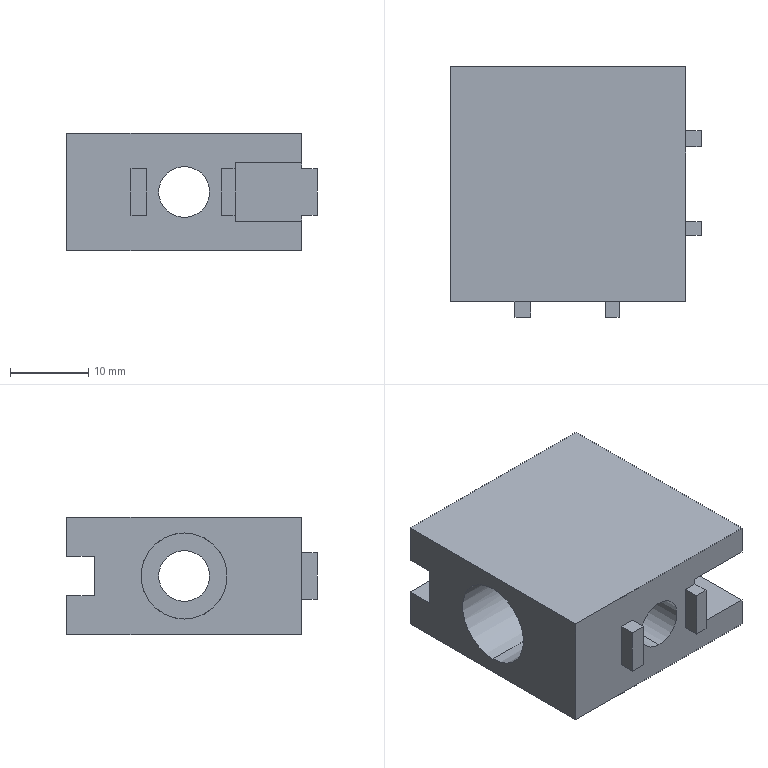Part | NX | features BREP 1 | 1 solid | 49 faces | box 32 x 32 x 15 mm | volume 8511 mm3 | plane 37 | cylinder 12 | commonest cylinder face diameters 11 x8 6.5 x4
STEP:
#1=CARTESIAN_POINT('',(0.,0.,5.5));
#2=VERTEX_POINT('',#1);
#3=CARTESIAN_POINT('',(0.,0.,-5.5));
#4=VERTEX_POINT('',#3);
#5=CARTESIAN_POINT('',(0.,0.,5.5));
#6=CARTESIAN_POINT('',(-11.,-11.,5.5));
#7=CARTESIAN_POINT('',(-11.,-11.,-5.5));
#8=CARTESIAN_POINT('',(0.,0.,-5.5));
#9=(BOUNDED_CURVE()B_SPLINE_CURVE(3,(#5,#6,#7,#8),.UNSPECIFIED.,.F.,.F.)B_SPLINE_CURVE_WITH_KNOTS((4,4),(4.712,7.854),.UNSPECIFIED.)CURVE()GEOMETRIC_REPRESENTATION_ITEM()RATIONAL_B_SPLINE_CURVE((1.,0.3333,0.3333,1.))REPRESENTATION_ITEM(''));
#10=EDGE_CURVE('',#2,#4,#9,.T.);
#11=ORIENTED_EDGE('',*,*,#10,.T.);
#12=CARTESIAN_POINT('',(-15.,0.,-5.5));
#13=VERTEX_POINT('',#12);
#14=CARTESIAN_POINT('',(0.,0.,-5.5));
#15=DIRECTION('',(-1.,0.,0.));
#16=VECTOR('',#15,1000.);
#17=LINE('',#14,#16);
#18=EDGE_CURVE('',#13,#4,#17,.F.);
#19=ORIENTED_EDGE('',*,*,#18,.F.);
#20=CARTESIAN_POINT('',(-15.,0.,5.5));
#21=VERTEX_POINT('',#20);
#22=CARTESIAN_POINT('',(-15.,0.,0.));
#23=DIRECTION('',(-1.,0.,0.));
#24=DIRECTION('',(0.,0.,1.));
#25=AXIS2_PLACEMENT_3D('',#22,#23,#24);
#26=CIRCLE('',#25,5.5);
#27=EDGE_CURVE('',#13,#21,#26,.T.);
#28=ORIENTED_EDGE('',*,*,#27,.T.);
#29=CARTESIAN_POINT('',(0.,0.,5.5));
#30=DIRECTION('',(-1.,0.,0.));
#31=VECTOR('',#30,1000.);
#32=LINE('',#29,#31);
#33=EDGE_CURVE('',#21,#2,#32,.F.);
#34=ORIENTED_EDGE('',*,*,#33,.T.);
#35=EDGE_LOOP('',(#11,#19,#28,#34));
#36=FACE_BOUND('',#35,.T.);
#37=CARTESIAN_POINT('',(0.,0.,0.));
#38=DIRECTION('',(-1.,0.,0.));
#39=DIRECTION('',(0.,0.,1.));
#40=AXIS2_PLACEMENT_3D('',#37,#38,#39);
#41=CYLINDRICAL_SURFACE('',#40,5.5);
#42=ADVANCED_FACE('',(#36),#41,.F.);
#43=CARTESIAN_POINT('',(10.,0.,-5.5));
#44=VERTEX_POINT('',#43);
#45=CARTESIAN_POINT('',(10.,0.,5.5));
#46=VERTEX_POINT('',#45);
#47=CARTESIAN_POINT('',(10.,0.,0.));
#48=DIRECTION('',(-1.,0.,0.));
#49=DIRECTION('',(0.,0.,1.));
#50=AXIS2_PLACEMENT_3D('',#47,#48,#49);
#51=CIRCLE('',#50,5.5);
#52=EDGE_CURVE('',#44,#46,#51,.T.);
#53=ORIENTED_EDGE('',*,*,#52,.F.);
#54=CARTESIAN_POINT('',(0.,0.,-5.5));
#55=DIRECTION('',(-1.,0.,0.));
#56=VECTOR('',#55,1000.);
#57=LINE('',#54,#56);
#58=EDGE_CURVE('',#4,#44,#57,.F.);
#59=ORIENTED_EDGE('',*,*,#58,.F.);
#60=CARTESIAN_POINT('',(0.,0.,-5.5));
#61=CARTESIAN_POINT('',(11.,-11.,-5.5));
#62=CARTESIAN_POINT('',(11.,-11.,5.5));
#63=CARTESIAN_POINT('',(0.,0.,5.5));
#64=(BOUNDED_CURVE()B_SPLINE_CURVE(3,(#60,#61,#62,#63),.UNSPECIFIED.,.F.,.F.)B_SPLINE_CURVE_WITH_KNOTS((4,4),(4.712,7.854),.UNSPECIFIED.)CURVE()GEOMETRIC_REPRESENTATION_ITEM()RATIONAL_B_SPLINE_CURVE((1.,0.3333,0.3333,1.))REPRESENTATION_ITEM(''));
#65=EDGE_CURVE('',#4,#2,#64,.T.);
#66=ORIENTED_EDGE('',*,*,#65,.T.);
#67=CARTESIAN_POINT('',(0.,0.,5.5));
#68=DIRECTION('',(-1.,0.,0.));
#69=VECTOR('',#68,1000.);
#70=LINE('',#67,#69);
#71=EDGE_CURVE('',#2,#46,#70,.F.);
#72=ORIENTED_EDGE('',*,*,#71,.T.);
#73=EDGE_LOOP('',(#53,#59,#66,#72));
#74=FACE_BOUND('',#73,.T.);
#75=CARTESIAN_POINT('',(0.,0.,0.));
#76=DIRECTION('',(-1.,0.,0.));
#77=DIRECTION('',(0.,0.,1.));
#78=AXIS2_PLACEMENT_3D('',#75,#76,#77);
#79=CYLINDRICAL_SURFACE('',#78,5.5);
#80=ADVANCED_FACE('',(#74),#79,.F.);
#81=CARTESIAN_POINT('',(15.,0.,-3.25));
#82=VERTEX_POINT('',#81);
#83=CARTESIAN_POINT('',(15.,0.,3.25));
#84=VERTEX_POINT('',#83);
#85=CARTESIAN_POINT('',(15.,0.,0.));
#86=DIRECTION('',(-1.,0.,0.));
#87=DIRECTION('',(0.,0.,1.));
#88=AXIS2_PLACEMENT_3D('',#85,#86,#87);
#89=CIRCLE('',#88,3.25);
#90=EDGE_CURVE('',#82,#84,#89,.T.);
#91=ORIENTED_EDGE('',*,*,#90,.F.);
#92=CARTESIAN_POINT('',(10.,0.,-3.25));
#93=VERTEX_POINT('',#92);
#94=CARTESIAN_POINT('',(0.,0.,-3.25));
#95=DIRECTION('',(-1.,0.,0.));
#96=VECTOR('',#95,1000.);
#97=LINE('',#94,#96);
#98=EDGE_CURVE('',#93,#82,#97,.F.);
#99=ORIENTED_EDGE('',*,*,#98,.F.);
#100=CARTESIAN_POINT('',(10.,0.,3.25));
#101=VERTEX_POINT('',#100);
#102=CARTESIAN_POINT('',(10.,0.,0.));
#103=DIRECTION('',(-1.,0.,0.));
#104=DIRECTION('',(0.,0.,1.));
#105=AXIS2_PLACEMENT_3D('',#102,#103,#104);
#106=CIRCLE('',#105,3.25);
#107=EDGE_CURVE('',#93,#101,#106,.T.);
#108=ORIENTED_EDGE('',*,*,#107,.T.);
#109=CARTESIAN_POINT('',(0.,0.,3.25));
#110=DIRECTION('',(-1.,0.,0.));
#111=VECTOR('',#110,1000.);
#112=LINE('',#109,#111);
#113=EDGE_CURVE('',#101,#84,#112,.F.);
#114=ORIENTED_EDGE('',*,*,#113,.T.);
#115=EDGE_LOOP('',(#91,#99,#108,#114));
#116=FACE_BOUND('',#115,.T.);
#117=CARTESIAN_POINT('',(0.,0.,0.));
#118=DIRECTION('',(-1.,0.,0.));
#119=DIRECTION('',(0.,0.,1.));
#120=AXIS2_PLACEMENT_3D('',#117,#118,#119);
#121=CYLINDRICAL_SURFACE('',#120,3.25);
#122=ADVANCED_FACE('',(#116),#121,.F.);
#123=CARTESIAN_POINT('',(0.,-10.,3.25));
#124=VERTEX_POINT('',#123);
#125=CARTESIAN_POINT('',(0.,-10.,-3.25));
#126=VERTEX_POINT('',#125);
#127=CARTESIAN_POINT('',(0.,-10.,0.));
#128=DIRECTION('',(0.,-1.,0.));
#129=DIRECTION('',(0.,0.,-1.));
#130=AXIS2_PLACEMENT_3D('',#127,#128,#129);
#131=CIRCLE('',#130,3.25);
#132=EDGE_CURVE('',#124,#126,#131,.T.);
#133=ORIENTED_EDGE('',*,*,#132,.F.);
#134=CARTESIAN_POINT('',(0.,-15.,3.25));
#135=VERTEX_POINT('',#134);
#136=CARTESIAN_POINT('',(0.,0.,3.25));
#137=DIRECTION('',(0.,-1.,0.));
#138=VECTOR('',#137,1000.);
#139=LINE('',#136,#138);
#140=EDGE_CURVE('',#124,#135,#139,.T.);
#141=ORIENTED_EDGE('',*,*,#140,.T.);
#142=CARTESIAN_POINT('',(0.,-15.,-3.25));
#143=VERTEX_POINT('',#142);
#144=CARTESIAN_POINT('',(0.,-15.,0.));
#145=DIRECTION('',(0.,-1.,0.));
#146=DIRECTION('',(0.,0.,-1.));
#147=AXIS2_PLACEMENT_3D('',#144,#145,#146);
#148=CIRCLE('',#147,3.25);
#149=EDGE_CURVE('',#135,#143,#148,.T.);
#150=ORIENTED_EDGE('',*,*,#149,.T.);
#151=CARTESIAN_POINT('',(0.,0.,-3.25));
#152=DIRECTION('',(0.,-1.,0.));
#153=VECTOR('',#152,1000.);
#154=LINE('',#151,#153);
#155=EDGE_CURVE('',#126,#143,#154,.T.);
#156=ORIENTED_EDGE('',*,*,#155,.F.);
#157=EDGE_LOOP('',(#133,#141,#150,#156));
#158=FACE_BOUND('',#157,.T.);
#159=CARTESIAN_POINT('',(0.,0.,0.));
#160=DIRECTION('',(0.,-1.,0.));
#161=DIRECTION('',(0.,0.,-1.));
#162=AXIS2_PLACEMENT_3D('',#159,#160,#161);
#163=CYLINDRICAL_SURFACE('',#162,3.25);
#164=ADVANCED_FACE('',(#158),#163,.F.);
#165=ORIENTED_EDGE('',*,*,#10,.F.);
#166=CARTESIAN_POINT('',(0.,-10.,5.5));
#167=VERTEX_POINT('',#166);
#168=CARTESIAN_POINT('',(0.,0.,5.5));
#169=DIRECTION('',(0.,-1.,0.));
#170=VECTOR('',#169,1000.);
#171=LINE('',#168,#170);
#172=EDGE_CURVE('',#2,#167,#171,.T.);
#173=ORIENTED_EDGE('',*,*,#172,.T.);
#174=CARTESIAN_POINT('',(0.,-10.,-5.5));
#175=VERTEX_POINT('',#174);
#176=CARTESIAN_POINT('',(0.,-10.,0.));
#177=DIRECTION('',(0.,-1.,0.));
#178=DIRECTION('',(0.,0.,-1.));
#179=AXIS2_PLACEMENT_3D('',#176,#177,#178);
#180=CIRCLE('',#179,5.5);
#181=EDGE_CURVE('',#167,#175,#180,.T.);
#182=ORIENTED_EDGE('',*,*,#181,.T.);
#183=CARTESIAN_POINT('',(0.,0.,-5.5));
#184=DIRECTION('',(0.,-1.,0.));
#185=VECTOR('',#184,1000.);
#186=LINE('',#183,#185);
#187=EDGE_CURVE('',#4,#175,#186,.T.);
#188=ORIENTED_EDGE('',*,*,#187,.F.);
#189=EDGE_LOOP('',(#165,#173,#182,#188));
#190=FACE_BOUND('',#189,.T.);
#191=CARTESIAN_POINT('',(0.,0.,0.));
#192=DIRECTION('',(0.,-1.,0.));
#193=DIRECTION('',(0.,0.,-1.));
#194=AXIS2_PLACEMENT_3D('',#191,#192,#193);
#195=CYLINDRICAL_SURFACE('',#194,5.5);
#196=ADVANCED_FACE('',(#190),#195,.F.);
#197=CARTESIAN_POINT('',(0.,15.,5.5));
#198=VERTEX_POINT('',#197);
#199=CARTESIAN_POINT('',(-4.899,15.,2.5));
#200=VERTEX_POINT('',#199);
#201=CARTESIAN_POINT('',(0.,15.,0.));
#202=DIRECTION('',(0.,-1.,0.));
#203=DIRECTION('',(0.,0.,-1.));
#204=AXIS2_PLACEMENT_3D('',#201,#202,#203);
#205=CIRCLE('',#204,5.5);
#206=EDGE_CURVE('',#198,#200,#205,.T.);
#207=ORIENTED_EDGE('',*,*,#206,.F.);
#208=CARTESIAN_POINT('',(0.,0.,5.5));
#209=DIRECTION('',(0.,-1.,0.));
#210=VECTOR('',#209,1000.);
#211=LINE('',#208,#210);
#212=EDGE_CURVE('',#198,#2,#211,.T.);
#213=ORIENTED_EDGE('',*,*,#212,.T.);
#214=CARTESIAN_POINT('',(0.,0.,-5.5));
#215=CARTESIAN_POINT('',(-11.,11.,-5.5));
#216=CARTESIAN_POINT('',(-11.,11.,5.5));
#217=CARTESIAN_POINT('',(0.,0.,5.5));
#218=(BOUNDED_CURVE()B_SPLINE_CURVE(3,(#214,#215,#216,#217),.UNSPECIFIED.,.F.,.F.)B_SPLINE_CURVE_WITH_KNOTS((4,4),(1.571,4.712),.UNSPECIFIED.)CURVE()GEOMETRIC_REPRESENTATION_ITEM()RATIONAL_B_SPLINE_CURVE((1.,0.3333,0.3333,1.))REPRESENTATION_ITEM(''));
#219=EDGE_CURVE('',#4,#2,#218,.T.);
#220=ORIENTED_EDGE('',*,*,#219,.F.);
#221=CARTESIAN_POINT('',(0.,15.,-5.5));
#222=VERTEX_POINT('',#221);
#223=CARTESIAN_POINT('',(0.,0.,-5.5));
#224=DIRECTION('',(0.,-1.,0.));
#225=VECTOR('',#224,1000.);
#226=LINE('',#223,#225);
#227=EDGE_CURVE('',#222,#4,#226,.T.);
#228=ORIENTED_EDGE('',*,*,#227,.F.);
#229=CARTESIAN_POINT('',(-4.899,15.,-2.5));
#230=VERTEX_POINT('',#229);
#231=CARTESIAN_POINT('',(0.,15.,0.));
#232=DIRECTION('',(0.,-1.,0.));
#233=DIRECTION('',(0.,0.,-1.));
#234=AXIS2_PLACEMENT_3D('',#231,#232,#233);
#235=CIRCLE('',#234,5.5);
#236=EDGE_CURVE('',#230,#222,#235,.T.);
#237=ORIENTED_EDGE('',*,*,#236,.F.);
#238=CARTESIAN_POINT('',(-4.899,11.5,-2.5));
#239=VERTEX_POINT('',#238);
#240=CARTESIAN_POINT('',(-4.899,0.,-2.5));
#241=DIRECTION('',(0.,-1.,0.));
#242=VECTOR('',#241,1000.);
#243=LINE('',#240,#242);
#244=EDGE_CURVE('',#230,#239,#243,.T.);
#245=ORIENTED_EDGE('',*,*,#244,.T.);
#246=CARTESIAN_POINT('',(-4.899,11.5,2.5));
#247=VERTEX_POINT('',#246);
#248=CARTESIAN_POINT('',(0.,11.5,0.));
#249=DIRECTION('',(0.,1.,0.));
#250=DIRECTION('',(0.,0.,-1.));
#251=AXIS2_PLACEMENT_3D('',#248,#249,#250);
#252=CIRCLE('',#251,5.5);
#253=EDGE_CURVE('',#239,#247,#252,.T.);
#254=ORIENTED_EDGE('',*,*,#253,.T.);
#255=CARTESIAN_POINT('',(-4.899,0.,2.5));
#256=DIRECTION('',(0.,1.,0.));
#257=VECTOR('',#256,1000.);
#258=LINE('',#255,#257);
#259=EDGE_CURVE('',#247,#200,#258,.T.);
#260=ORIENTED_EDGE('',*,*,#259,.T.);
#261=EDGE_LOOP('',(#207,#213,#220,#228,#237,#245,#254,#260));
#262=FACE_BOUND('',#261,.T.);
#263=CARTESIAN_POINT('',(0.,0.,0.));
#264=DIRECTION('',(0.,-1.,0.));
#265=DIRECTION('',(0.,0.,-1.));
#266=AXIS2_PLACEMENT_3D('',#263,#264,#265);
#267=CYLINDRICAL_SURFACE('',#266,5.5);
#268=ADVANCED_FACE('',(#262),#267,.F.);
#269=CARTESIAN_POINT('',(-15.,15.,2.5));
#270=VERTEX_POINT('',#269);
#271=CARTESIAN_POINT('',(-15.,15.,2.5));
#272=DIRECTION('',(1.,0.,0.));
#273=VECTOR('',#272,1000.);
#274=LINE('',#271,#273);
#275=EDGE_CURVE('',#270,#200,#274,.T.);
#276=ORIENTED_EDGE('',*,*,#275,.F.);
#277=CARTESIAN_POINT('',(-15.,15.,7.5));
#278=VERTEX_POINT('',#277);
#279=CARTESIAN_POINT('',(-15.,15.,-7.5));
#280=DIRECTION('',(0.,0.,1.));
#281=VECTOR('',#280,1000.);
#282=LINE('',#279,#281);
#283=EDGE_CURVE('',#270,#278,#282,.T.);
#284=ORIENTED_EDGE('',*,*,#283,.T.);
#285=CARTESIAN_POINT('',(15.,15.,7.5));
#286=VERTEX_POINT('',#285);
#287=CARTESIAN_POINT('',(-15.,15.,7.5));
#288=DIRECTION('',(-1.,0.,0.));
#289=VECTOR('',#288,1000.);
#290=LINE('',#287,#289);
#291=EDGE_CURVE('',#286,#278,#290,.T.);
#292=ORIENTED_EDGE('',*,*,#291,.F.);
#293=CARTESIAN_POINT('',(15.,15.,2.5));
#294=VERTEX_POINT('',#293);
#295=CARTESIAN_POINT('',(15.,15.,-7.5));
#296=DIRECTION('',(0.,0.,1.));
#297=VECTOR('',#296,1000.);
#298=LINE('',#295,#297);
#299=EDGE_CURVE('',#294,#286,#298,.T.);
#300=ORIENTED_EDGE('',*,*,#299,.F.);
#301=CARTESIAN_POINT('',(4.899,15.,2.5));
#302=VERTEX_POINT('',#301);
#303=CARTESIAN_POINT('',(-15.,15.,2.5));
#304=DIRECTION('',(1.,0.,0.));
#305=VECTOR('',#304,1000.);
#306=LINE('',#303,#305);
#307=EDGE_CURVE('',#302,#294,#306,.T.);
#308=ORIENTED_EDGE('',*,*,#307,.F.);
#309=CARTESIAN_POINT('',(0.,15.,0.));
#310=DIRECTION('',(0.,-1.,0.));
#311=DIRECTION('',(0.,0.,-1.));
#312=AXIS2_PLACEMENT_3D('',#309,#310,#311);
#313=CIRCLE('',#312,5.5);
#314=EDGE_CURVE('',#302,#198,#313,.T.);
#315=ORIENTED_EDGE('',*,*,#314,.T.);
#316=ORIENTED_EDGE('',*,*,#206,.T.);
#317=EDGE_LOOP('',(#276,#284,#292,#300,#308,#315,#316));
#318=FACE_BOUND('',#317,.T.);
#319=CARTESIAN_POINT('',(-15.,15.,-7.5));
#320=DIRECTION('',(0.,1.,0.));
#321=DIRECTION('',(1.,0.,0.));
#322=AXIS2_PLACEMENT_3D('',#319,#320,#321);
#323=PLANE('',#322);
#324=ADVANCED_FACE('',(#318),#323,.T.);
#325=CARTESIAN_POINT('',(15.,-6.5,-3.75));
#326=VERTEX_POINT('',#325);
#327=CARTESIAN_POINT('',(15.,-6.5,-3.));
#328=VERTEX_POINT('',#327);
#329=CARTESIAN_POINT('',(15.,-6.5,-3.75));
#330=DIRECTION('',(0.,0.,1.));
#331=VECTOR('',#330,1000.);
#332=LINE('',#329,#331);
#333=EDGE_CURVE('',#326,#328,#332,.T.);
#334=ORIENTED_EDGE('',*,*,#333,.F.);
#335=CARTESIAN_POINT('',(15.,-15.,-3.75));
#336=VERTEX_POINT('',#335);
#337=CARTESIAN_POINT('',(15.,-6.5,-3.75));
#338=DIRECTION('',(0.,1.,0.));
#339=VECTOR('',#338,1000.);
#340=LINE('',#337,#339);
#341=EDGE_CURVE('',#336,#326,#340,.T.);
#342=ORIENTED_EDGE('',*,*,#341,.F.);
#343=CARTESIAN_POINT('',(15.,-15.,-7.5));
#344=VERTEX_POINT('',#343);
#345=CARTESIAN_POINT('',(15.,-15.,-7.5));
#346=DIRECTION('',(0.,0.,1.));
#347=VECTOR('',#346,1000.);
#348=LINE('',#345,#347);
#349=EDGE_CURVE('',#344,#336,#348,.T.);
#350=ORIENTED_EDGE('',*,*,#349,.F.);
#351=CARTESIAN_POINT('',(15.,15.,-7.5));
#352=VERTEX_POINT('',#351);
#353=CARTESIAN_POINT('',(15.,-15.,-7.5));
#354=DIRECTION('',(0.,1.,0.));
#355=VECTOR('',#354,1000.);
#356=LINE('',#353,#355);
#357=EDGE_CURVE('',#344,#352,#356,.T.);
#358=ORIENTED_EDGE('',*,*,#357,.T.);
#359=CARTESIAN_POINT('',(15.,15.,-2.5));
#360=VERTEX_POINT('',#359);
#361=CARTESIAN_POINT('',(15.,15.,-7.5));
#362=DIRECTION('',(0.,0.,1.));
#363=VECTOR('',#362,1000.);
#364=LINE('',#361,#363);
#365=EDGE_CURVE('',#352,#360,#364,.T.);
#366=ORIENTED_EDGE('',*,*,#365,.T.);
#367=CARTESIAN_POINT('',(15.,11.5,-2.5));
#368=VERTEX_POINT('',#367);
#369=CARTESIAN_POINT('',(15.,-15.,-2.5));
#370=DIRECTION('',(0.,1.,0.));
#371=VECTOR('',#370,1000.);
#372=LINE('',#369,#371);
#373=EDGE_CURVE('',#368,#360,#372,.T.);
#374=ORIENTED_EDGE('',*,*,#373,.F.);
#375=CARTESIAN_POINT('',(15.,11.5,2.5));
#376=VERTEX_POINT('',#375);
#377=CARTESIAN_POINT('',(15.,11.5,-7.5));
#378=DIRECTION('',(0.,0.,-1.));
#379=VECTOR('',#378,1000.);
#380=LINE('',#377,#379);
#381=EDGE_CURVE('',#376,#368,#380,.T.);
#382=ORIENTED_EDGE('',*,*,#381,.F.);
#383=CARTESIAN_POINT('',(15.,-15.,2.5));
#384=DIRECTION('',(0.,-1.,0.));
#385=VECTOR('',#384,1000.);
#386=LINE('',#383,#385);
#387=EDGE_CURVE('',#294,#376,#386,.T.);
#388=ORIENTED_EDGE('',*,*,#387,.F.);
#389=ORIENTED_EDGE('',*,*,#299,.T.);
#390=CARTESIAN_POINT('',(15.,-15.,7.5));
#391=VERTEX_POINT('',#390);
#392=CARTESIAN_POINT('',(15.,-15.,7.5));
#393=DIRECTION('',(0.,1.,0.));
#394=VECTOR('',#393,1000.);
#395=LINE('',#392,#394);
#396=EDGE_CURVE('',#391,#286,#395,.T.);
#397=ORIENTED_EDGE('',*,*,#396,.F.);
#398=CARTESIAN_POINT('',(15.,-15.,3.75));
#399=VERTEX_POINT('',#398);
#400=CARTESIAN_POINT('',(15.,-15.,-7.5));
#401=DIRECTION('',(0.,0.,1.));
#402=VECTOR('',#401,1000.);
#403=LINE('',#400,#402);
#404=EDGE_CURVE('',#399,#391,#403,.T.);
#405=ORIENTED_EDGE('',*,*,#404,.F.);
#406=CARTESIAN_POINT('',(15.,-6.5,3.75));
#407=VERTEX_POINT('',#406);
#408=CARTESIAN_POINT('',(15.,-6.5,3.75));
#409=DIRECTION('',(0.,1.,0.));
#410=VECTOR('',#409,1000.);
#411=LINE('',#408,#410);
#412=EDGE_CURVE('',#399,#407,#411,.T.);
#413=ORIENTED_EDGE('',*,*,#412,.T.);
#414=CARTESIAN_POINT('',(15.,-6.5,3.));
#415=VERTEX_POINT('',#414);
#416=CARTESIAN_POINT('',(15.,-6.5,-3.75));
#417=DIRECTION('',(0.,0.,1.));
#418=VECTOR('',#417,1000.);
#419=LINE('',#416,#418);
#420=EDGE_CURVE('',#415,#407,#419,.T.);
#421=ORIENTED_EDGE('',*,*,#420,.F.);
#422=CARTESIAN_POINT('',(15.,-4.8,3.));
#423=VERTEX_POINT('',#422);
#424=CARTESIAN_POINT('',(15.,-4.8,3.));
#425=DIRECTION('',(0.,-1.,0.));
#426=VECTOR('',#425,1000.);
#427=LINE('',#424,#426);
#428=EDGE_CURVE('',#423,#415,#427,.T.);
#429=ORIENTED_EDGE('',*,*,#428,.F.);
#430=CARTESIAN_POINT('',(15.,-4.8,-3.));
#431=VERTEX_POINT('',#430);
#432=CARTESIAN_POINT('',(15.,-4.8,3.));
#433=DIRECTION('',(0.,0.,1.));
#434=VECTOR('',#433,1000.);
#435=LINE('',#432,#434);
#436=EDGE_CURVE('',#431,#423,#435,.T.);
#437=ORIENTED_EDGE('',*,*,#436,.F.);
#438=CARTESIAN_POINT('',(15.,-4.8,-3.));
#439=DIRECTION('',(0.,1.,0.));
#440=VECTOR('',#439,1000.);
#441=LINE('',#438,#440);
#442=EDGE_CURVE('',#328,#431,#441,.T.);
#443=ORIENTED_EDGE('',*,*,#442,.F.);
#444=EDGE_LOOP('',(#334,#342,#350,#358,#366,#374,#382,#388,#389,#397,#405,#413,#421,#429,#437,#443));
#445=FACE_BOUND('',#444,.T.);
#446=CARTESIAN_POINT('',(15.,6.8,-3.));
#447=VERTEX_POINT('',#446);
#448=CARTESIAN_POINT('',(15.,6.8,3.));
#449=VERTEX_POINT('',#448);
#450=CARTESIAN_POINT('',(15.,6.8,3.));
#451=DIRECTION('',(0.,0.,1.));
#452=VECTOR('',#451,1000.);
#453=LINE('',#450,#452);
#454=EDGE_CURVE('',#447,#449,#453,.T.);
#455=ORIENTED_EDGE('',*,*,#454,.F.);
#456=CARTESIAN_POINT('',(15.,4.8,-3.));
#457=VERTEX_POINT('',#456);
#458=CARTESIAN_POINT('',(15.,6.8,-3.));
#459=DIRECTION('',(0.,1.,0.));
#460=VECTOR('',#459,1000.);
#461=LINE('',#458,#460);
#462=EDGE_CURVE('',#457,#447,#461,.T.);
#463=ORIENTED_EDGE('',*,*,#462,.F.);
#464=CARTESIAN_POINT('',(15.,4.8,3.));
#465=VERTEX_POINT('',#464);
#466=CARTESIAN_POINT('',(15.,4.8,3.));
#467=DIRECTION('',(0.,0.,-1.));
#468=VECTOR('',#467,1000.);
#469=LINE('',#466,#468);
#470=EDGE_CURVE('',#465,#457,#469,.T.);
#471=ORIENTED_EDGE('',*,*,#470,.F.);
#472=CARTESIAN_POINT('',(15.,6.8,3.));
#473=DIRECTION('',(0.,-1.,0.));
#474=VECTOR('',#473,1000.);
#475=LINE('',#472,#474);
#476=EDGE_CURVE('',#449,#465,#475,.T.);
#477=ORIENTED_EDGE('',*,*,#476,.F.);
#478=EDGE_LOOP('',(#455,#463,#471,#477));
#479=FACE_BOUND('',#478,.T.);
#480=CARTESIAN_POINT('',(15.,0.,0.));
#481=DIRECTION('',(-1.,0.,0.));
#482=DIRECTION('',(0.,0.,1.));
#483=AXIS2_PLACEMENT_3D('',#480,#481,#482);
#484=CIRCLE('',#483,3.25);
#485=EDGE_CURVE('',#84,#82,#484,.T.);
#486=ORIENTED_EDGE('',*,*,#485,.T.);
#487=ORIENTED_EDGE('',*,*,#90,.T.);
#488=EDGE_LOOP('',(#486,#487));
#489=FACE_BOUND('',#488,.T.);
#490=CARTESIAN_POINT('',(15.,-15.,-7.5));
#491=DIRECTION('',(1.,0.,0.));
#492=DIRECTION('',(0.,1.,0.));
#493=AXIS2_PLACEMENT_3D('',#490,#491,#492);
#494=PLANE('',#493);
#495=ADVANCED_FACE('',(#445,#479,#489),#494,.T.);
#496=CARTESIAN_POINT('',(6.5,-15.,-3.75));
#497=VERTEX_POINT('',#496);
#498=CARTESIAN_POINT('',(6.5,-15.,-3.));
#499=VERTEX_POINT('',#498);
#500=CARTESIAN_POINT('',(6.5,-15.,-3.75));
#501=DIRECTION('',(0.,0.,1.));
#502=VECTOR('',#501,1000.);
#503=LINE('',#500,#502);
#504=EDGE_CURVE('',#497,#499,#503,.T.);
#505=ORIENTED_EDGE('',*,*,#504,.T.);
#506=CARTESIAN_POINT('',(4.8,-15.,-3.));
#507=VERTEX_POINT('',#506);
#508=CARTESIAN_POINT('',(4.8,-15.,-3.));
#509=DIRECTION('',(1.,0.,0.));
#510=VECTOR('',#509,1000.);
#511=LINE('',#508,#510);
#512=EDGE_CURVE('',#507,#499,#511,.T.);
#513=ORIENTED_EDGE('',*,*,#512,.F.);
#514=CARTESIAN_POINT('',(4.8,-15.,3.));
#515=VERTEX_POINT('',#514);
#516=CARTESIAN_POINT('',(4.8,-15.,3.));
#517=DIRECTION('',(0.,0.,-1.));
#518=VECTOR('',#517,1000.);
#519=LINE('',#516,#518);
#520=EDGE_CURVE('',#515,#507,#519,.T.);
#521=ORIENTED_EDGE('',*,*,#520,.F.);
#522=CARTESIAN_POINT('',(6.5,-15.,3.));
#523=VERTEX_POINT('',#522);
#524=CARTESIAN_POINT('',(4.8,-15.,3.));
#525=DIRECTION('',(-1.,0.,0.));
#526=VECTOR('',#525,1000.);
#527=LINE('',#524,#526);
#528=EDGE_CURVE('',#523,#515,#527,.T.);
#529=ORIENTED_EDGE('',*,*,#528,.F.);
#530=CARTESIAN_POINT('',(6.5,-15.,3.75));
#531=VERTEX_POINT('',#530);
#532=CARTESIAN_POINT('',(6.5,-15.,-3.75));
#533=DIRECTION('',(0.,0.,1.));
#534=VECTOR('',#533,1000.);
#535=LINE('',#532,#534);
#536=EDGE_CURVE('',#523,#531,#535,.T.);
#537=ORIENTED_EDGE('',*,*,#536,.T.);
#538=CARTESIAN_POINT('',(6.5,-15.,3.75));
#539=DIRECTION('',(1.,0.,0.));
#540=VECTOR('',#539,1000.);
#541=LINE('',#538,#540);
#542=EDGE_CURVE('',#531,#399,#541,.T.);
#543=ORIENTED_EDGE('',*,*,#542,.T.);
#544=ORIENTED_EDGE('',*,*,#404,.T.);
#545=CARTESIAN_POINT('',(-15.,-15.,7.5));
#546=VERTEX_POINT('',#545);
#547=CARTESIAN_POINT('',(-15.,-15.,7.5));
#548=DIRECTION('',(1.,0.,0.));
#549=VECTOR('',#548,1000.);
#550=LINE('',#547,#549);
#551=EDGE_CURVE('',#546,#391,#550,.T.);
#552=ORIENTED_EDGE('',*,*,#551,.F.);
#553=CARTESIAN_POINT('',(-15.,-15.,-7.5));
#554=VERTEX_POINT('',#553);
#555=CARTESIAN_POINT('',(-15.,-15.,-7.5));
#556=DIRECTION('',(0.,0.,1.));
#557=VECTOR('',#556,1000.);
#558=LINE('',#555,#557);
#559=EDGE_CURVE('',#554,#546,#558,.T.);
#560=ORIENTED_EDGE('',*,*,#559,.F.);
#561=CARTESIAN_POINT('',(-15.,-15.,-7.5));
#562=DIRECTION('',(1.,0.,0.));
#563=VECTOR('',#562,1000.);
#564=LINE('',#561,#563);
#565=EDGE_CURVE('',#554,#344,#564,.T.);
#566=ORIENTED_EDGE('',*,*,#565,.T.);
#567=ORIENTED_EDGE('',*,*,#349,.T.);
#568=CARTESIAN_POINT('',(6.5,-15.,-3.75));
#569=DIRECTION('',(1.,0.,0.));
#570=VECTOR('',#569,1000.);
#571=LINE('',#568,#570);
#572=EDGE_CURVE('',#497,#336,#571,.T.);
#573=ORIENTED_EDGE('',*,*,#572,.F.);
#574=EDGE_LOOP('',(#505,#513,#521,#529,#537,#543,#544,#552,#560,#566,#567,#573));
#575=FACE_BOUND('',#574,.T.);
#576=CARTESIAN_POINT('',(-4.8,-15.,3.));
#577=VERTEX_POINT('',#576);
#578=CARTESIAN_POINT('',(-6.8,-15.,3.));
#579=VERTEX_POINT('',#578);
#580=CARTESIAN_POINT('',(-6.8,-15.,3.));
#581=DIRECTION('',(-1.,0.,0.));
#582=VECTOR('',#581,1000.);
#583=LINE('',#580,#582);
#584=EDGE_CURVE('',#577,#579,#583,.T.);
#585=ORIENTED_EDGE('',*,*,#584,.F.);
#586=CARTESIAN_POINT('',(-4.8,-15.,-3.));
#587=VERTEX_POINT('',#586);
#588=CARTESIAN_POINT('',(-4.8,-15.,3.));
#589=DIRECTION('',(0.,0.,1.));
#590=VECTOR('',#589,1000.);
#591=LINE('',#588,#590);
#592=EDGE_CURVE('',#587,#577,#591,.T.);
#593=ORIENTED_EDGE('',*,*,#592,.F.);
#594=CARTESIAN_POINT('',(-6.8,-15.,-3.));
#595=VERTEX_POINT('',#594);
#596=CARTESIAN_POINT('',(-6.8,-15.,-3.));
#597=DIRECTION('',(1.,0.,0.));
#598=VECTOR('',#597,1000.);
#599=LINE('',#596,#598);
#600=EDGE_CURVE('',#595,#587,#599,.T.);
#601=ORIENTED_EDGE('',*,*,#600,.F.);
#602=CARTESIAN_POINT('',(-6.8,-15.,3.));
#603=DIRECTION('',(0.,0.,-1.));
#604=VECTOR('',#603,1000.);
#605=LINE('',#602,#604);
#606=EDGE_CURVE('',#579,#595,#605,.T.);
#607=ORIENTED_EDGE('',*,*,#606,.F.);
#608=EDGE_LOOP('',(#585,#593,#601,#607));
#609=FACE_BOUND('',#608,.T.);
#610=CARTESIAN_POINT('',(0.,-15.,0.));
#611=DIRECTION('',(0.,-1.,0.));
#612=DIRECTION('',(0.,0.,-1.));
#613=AXIS2_PLACEMENT_3D('',#610,#611,#612);
#614=CIRCLE('',#613,3.25);
#615=EDGE_CURVE('',#143,#135,#614,.T.);
#616=ORIENTED_EDGE('',*,*,#615,.F.);
#617=ORIENTED_EDGE('',*,*,#149,.F.);
#618=EDGE_LOOP('',(#616,#617));
#619=FACE_BOUND('',#618,.T.);
#620=CARTESIAN_POINT('',(-15.,-15.,-7.5));
#621=DIRECTION('',(0.,-1.,0.));
#622=DIRECTION('',(0.,0.,-1.));
#623=AXIS2_PLACEMENT_3D('',#620,#621,#622);
#624=PLANE('',#623);
#625=ADVANCED_FACE('',(#575,#609,#619),#624,.T.);
#626=CARTESIAN_POINT('',(-15.,11.5,2.5));
#627=VERTEX_POINT('',#626);
#628=CARTESIAN_POINT('',(-15.,11.5,2.5));
#629=DIRECTION('',(0.,1.,0.));
#630=VECTOR('',#629,1000.);
#631=LINE('',#628,#630);
#632=EDGE_CURVE('',#627,#270,#631,.T.);
#633=ORIENTED_EDGE('',*,*,#632,.F.);
#634=CARTESIAN_POINT('',(-15.,11.5,-2.5));
#635=VERTEX_POINT('',#634);
#636=CARTESIAN_POINT('',(-15.,11.5,-2.5));
#637=DIRECTION('',(0.,0.,1.));
#638=VECTOR('',#637,1000.);
#639=LINE('',#636,#638);
#640=EDGE_CURVE('',#635,#627,#639,.T.);
#641=ORIENTED_EDGE('',*,*,#640,.F.);
#642=CARTESIAN_POINT('',(-15.,15.,-2.5));
#643=VERTEX_POINT('',#642);
#644=CARTESIAN_POINT('',(-15.,11.5,-2.5));
#645=DIRECTION('',(0.,-1.,0.));
#646=VECTOR('',#645,1000.);
#647=LINE('',#644,#646);
#648=EDGE_CURVE('',#643,#635,#647,.T.);
#649=ORIENTED_EDGE('',*,*,#648,.F.);
#650=CARTESIAN_POINT('',(-15.,15.,-7.5));
#651=VERTEX_POINT('',#650);
#652=CARTESIAN_POINT('',(-15.,15.,-7.5));
#653=DIRECTION('',(0.,0.,1.));
#654=VECTOR('',#653,1000.);
#655=LINE('',#652,#654);
#656=EDGE_CURVE('',#651,#643,#655,.T.);
#657=ORIENTED_EDGE('',*,*,#656,.F.);
#658=CARTESIAN_POINT('',(-15.,-15.,-7.5));
#659=DIRECTION('',(0.,-1.,0.));
#660=VECTOR('',#659,1000.);
#661=LINE('',#658,#660);
#662=EDGE_CURVE('',#651,#554,#661,.T.);
#663=ORIENTED_EDGE('',*,*,#662,.T.);
#664=ORIENTED_EDGE('',*,*,#559,.T.);
#665=CARTESIAN_POINT('',(-15.,-15.,7.5));
#666=DIRECTION('',(0.,-1.,0.));
#667=VECTOR('',#666,1000.);
#668=LINE('',#665,#667);
#669=EDGE_CURVE('',#278,#546,#668,.T.);
#670=ORIENTED_EDGE('',*,*,#669,.F.);
#671=ORIENTED_EDGE('',*,*,#283,.F.);
#672=EDGE_LOOP('',(#633,#641,#649,#657,#663,#664,#670,#671));
#673=FACE_BOUND('',#672,.T.);
#674=CARTESIAN_POINT('',(-15.,0.,0.));
#675=DIRECTION('',(-1.,0.,0.));
#676=DIRECTION('',(0.,0.,1.));
#677=AXIS2_PLACEMENT_3D('',#674,#675,#676);
#678=CIRCLE('',#677,5.5);
#679=EDGE_CURVE('',#21,#13,#678,.T.);
#680=ORIENTED_EDGE('',*,*,#679,.F.);
#681=ORIENTED_EDGE('',*,*,#27,.F.);
#682=EDGE_LOOP('',(#680,#681));
#683=FACE_BOUND('',#682,.T.);
#684=CARTESIAN_POINT('',(-15.,-15.,-7.5));
#685=DIRECTION('',(-1.,0.,0.));
#686=DIRECTION('',(0.,0.,1.));
#687=AXIS2_PLACEMENT_3D('',#684,#685,#686);
#688=PLANE('',#687);
#689=ADVANCED_FACE('',(#673,#683),#688,.T.);
#690=ORIENTED_EDGE('',*,*,#212,.F.);
#691=ORIENTED_EDGE('',*,*,#314,.F.);
#692=CARTESIAN_POINT('',(4.899,11.5,2.5));
#693=VERTEX_POINT('',#692);
#694=CARTESIAN_POINT('',(4.899,0.,2.5));
#695=DIRECTION('',(0.,-1.,0.));
#696=VECTOR('',#695,1000.);
#697=LINE('',#694,#696);
#698=EDGE_CURVE('',#302,#693,#697,.T.);
#699=ORIENTED_EDGE('',*,*,#698,.T.);
#700=CARTESIAN_POINT('',(4.899,11.5,-2.5));
#701=VERTEX_POINT('',#700);
#702=CARTESIAN_POINT('',(0.,11.5,0.));
#703=DIRECTION('',(0.,1.,0.));
#704=DIRECTION('',(0.,0.,-1.));
#705=AXIS2_PLACEMENT_3D('',#702,#703,#704);
#706=CIRCLE('',#705,5.5);
#707=EDGE_CURVE('',#693,#701,#706,.T.);
#708=ORIENTED_EDGE('',*,*,#707,.T.);
#709=CARTESIAN_POINT('',(4.899,15.,-2.5));
#710=VERTEX_POINT('',#709);
#711=CARTESIAN_POINT('',(4.899,0.,-2.5));
#712=DIRECTION('',(0.,1.,0.));
#713=VECTOR('',#712,1000.);
#714=LINE('',#711,#713);
#715=EDGE_CURVE('',#701,#710,#714,.T.);
#716=ORIENTED_EDGE('',*,*,#715,.T.);
#717=CARTESIAN_POINT('',(0.,15.,0.));
#718=DIRECTION('',(0.,-1.,0.));
#719=DIRECTION('',(0.,0.,-1.));
#720=AXIS2_PLACEMENT_3D('',#717,#718,#719);
#721=CIRCLE('',#720,5.5);
#722=EDGE_CURVE('',#222,#710,#721,.T.);
#723=ORIENTED_EDGE('',*,*,#722,.F.);
#724=ORIENTED_EDGE('',*,*,#227,.T.);
#725=CARTESIAN_POINT('',(0.,0.,5.5));
#726=CARTESIAN_POINT('',(11.,11.,5.5));
#727=CARTESIAN_POINT('',(11.,11.,-5.5));
#728=CARTESIAN_POINT('',(0.,0.,-5.5));
#729=(BOUNDED_CURVE()B_SPLINE_CURVE(3,(#725,#726,#727,#728),.UNSPECIFIED.,.F.,.F.)B_SPLINE_CURVE_WITH_KNOTS((4,4),(1.571,4.712),.UNSPECIFIED.)CURVE()GEOMETRIC_REPRESENTATION_ITEM()RATIONAL_B_SPLINE_CURVE((1.,0.3333,0.3333,1.))REPRESENTATION_ITEM(''));
#730=EDGE_CURVE('',#2,#4,#729,.T.);
#731=ORIENTED_EDGE('',*,*,#730,.F.);
#732=EDGE_LOOP('',(#690,#691,#699,#708,#716,#723,#724,#731));
#733=FACE_BOUND('',#732,.T.);
#734=CARTESIAN_POINT('',(0.,0.,0.));
#735=DIRECTION('',(0.,-1.,0.));
#736=DIRECTION('',(0.,0.,-1.));
#737=AXIS2_PLACEMENT_3D('',#734,#735,#736);
#738=CYLINDRICAL_SURFACE('',#737,5.5);
#739=ADVANCED_FACE('',(#733),#738,.F.);
#740=ORIENTED_EDGE('',*,*,#172,.F.);
#741=ORIENTED_EDGE('',*,*,#65,.F.);
#742=ORIENTED_EDGE('',*,*,#187,.T.);
#743=CARTESIAN_POINT('',(0.,-10.,0.));
#744=DIRECTION('',(0.,-1.,0.));
#745=DIRECTION('',(0.,0.,-1.));
#746=AXIS2_PLACEMENT_3D('',#743,#744,#745);
#747=CIRCLE('',#746,5.5);
#748=EDGE_CURVE('',#175,#167,#747,.T.);
#749=ORIENTED_EDGE('',*,*,#748,.T.);
#750=EDGE_LOOP('',(#740,#741,#742,#749));
#751=FACE_BOUND('',#750,.T.);
#752=CARTESIAN_POINT('',(0.,0.,0.));
#753=DIRECTION('',(0.,-1.,0.));
#754=DIRECTION('',(0.,0.,-1.));
#755=AXIS2_PLACEMENT_3D('',#752,#753,#754);
#756=CYLINDRICAL_SURFACE('',#755,5.5);
#757=ADVANCED_FACE('',(#751),#756,.F.);
#758=CARTESIAN_POINT('',(-15.,15.,-2.5));
#759=DIRECTION('',(-1.,0.,0.));
#760=VECTOR('',#759,1000.);
#761=LINE('',#758,#760);
#762=EDGE_CURVE('',#360,#710,#761,.T.);
#763=ORIENTED_EDGE('',*,*,#762,.F.);
#764=ORIENTED_EDGE('',*,*,#365,.F.);
#765=CARTESIAN_POINT('',(-15.,15.,-7.5));
#766=DIRECTION('',(-1.,0.,0.));
#767=VECTOR('',#766,1000.);
#768=LINE('',#765,#767);
#769=EDGE_CURVE('',#352,#651,#768,.T.);
#770=ORIENTED_EDGE('',*,*,#769,.T.);
#771=ORIENTED_EDGE('',*,*,#656,.T.);
#772=CARTESIAN_POINT('',(-15.,15.,-2.5));
#773=DIRECTION('',(-1.,0.,0.));
#774=VECTOR('',#773,1000.);
#775=LINE('',#772,#774);
#776=EDGE_CURVE('',#230,#643,#775,.T.);
#777=ORIENTED_EDGE('',*,*,#776,.F.);
#778=ORIENTED_EDGE('',*,*,#236,.T.);
#779=ORIENTED_EDGE('',*,*,#722,.T.);
#780=EDGE_LOOP('',(#763,#764,#770,#771,#777,#778,#779));
#781=FACE_BOUND('',#780,.T.);
#782=CARTESIAN_POINT('',(-15.,15.,-7.5));
#783=DIRECTION('',(0.,1.,0.));
#784=DIRECTION('',(1.,0.,0.));
#785=AXIS2_PLACEMENT_3D('',#782,#783,#784);
#786=PLANE('',#785);
#787=ADVANCED_FACE('',(#781),#786,.T.);
#788=ORIENTED_EDGE('',*,*,#357,.F.);
#789=ORIENTED_EDGE('',*,*,#565,.F.);
#790=ORIENTED_EDGE('',*,*,#662,.F.);
#791=ORIENTED_EDGE('',*,*,#769,.F.);
#792=EDGE_LOOP('',(#788,#789,#790,#791));
#793=FACE_BOUND('',#792,.T.);
#794=CARTESIAN_POINT('',(0.,0.,-7.5));
#795=DIRECTION('',(0.,0.,-1.));
#796=DIRECTION('',(0.,-1.,0.));
#797=AXIS2_PLACEMENT_3D('',#794,#795,#796);
#798=PLANE('',#797);
#799=ADVANCED_FACE('',(#793),#798,.T.);
#800=ORIENTED_EDGE('',*,*,#396,.T.);
#801=ORIENTED_EDGE('',*,*,#291,.T.);
#802=ORIENTED_EDGE('',*,*,#669,.T.);
#803=ORIENTED_EDGE('',*,*,#551,.T.);
#804=EDGE_LOOP('',(#800,#801,#802,#803));
#805=FACE_BOUND('',#804,.T.);
#806=CARTESIAN_POINT('',(0.,0.,7.5));
#807=DIRECTION('',(0.,0.,-1.));
#808=DIRECTION('',(0.,-1.,0.));
#809=AXIS2_PLACEMENT_3D('',#806,#807,#808);
#810=PLANE('',#809);
#811=ADVANCED_FACE('',(#805),#810,.F.);
#812=ORIENTED_EDGE('',*,*,#748,.F.);
#813=ORIENTED_EDGE('',*,*,#181,.F.);
#814=EDGE_LOOP('',(#812,#813));
#815=FACE_BOUND('',#814,.T.);
#816=CARTESIAN_POINT('',(0.,-10.,0.));
#817=DIRECTION('',(0.,-1.,0.));
#818=DIRECTION('',(0.,0.,-1.));
#819=AXIS2_PLACEMENT_3D('',#816,#817,#818);
#820=CIRCLE('',#819,3.25);
#821=EDGE_CURVE('',#126,#124,#820,.T.);
#822=ORIENTED_EDGE('',*,*,#821,.T.);
#823=ORIENTED_EDGE('',*,*,#132,.T.);
#824=EDGE_LOOP('',(#822,#823));
#825=FACE_BOUND('',#824,.T.);
#826=CARTESIAN_POINT('',(5.5,-10.,0.));
#827=DIRECTION('',(0.,-1.,0.));
#828=DIRECTION('',(0.,0.,-1.));
#829=AXIS2_PLACEMENT_3D('',#826,#827,#828);
#830=PLANE('',#829);
#831=ADVANCED_FACE('',(#815,#825),#830,.F.);
#832=ORIENTED_EDGE('',*,*,#140,.F.);
#833=ORIENTED_EDGE('',*,*,#821,.F.);
#834=ORIENTED_EDGE('',*,*,#155,.T.);
#835=ORIENTED_EDGE('',*,*,#615,.T.);
#836=EDGE_LOOP('',(#832,#833,#834,#835));
#837=FACE_BOUND('',#836,.T.);
#838=CARTESIAN_POINT('',(0.,0.,0.));
#839=DIRECTION('',(0.,-1.,0.));
#840=DIRECTION('',(0.,0.,-1.));
#841=AXIS2_PLACEMENT_3D('',#838,#839,#840);
#842=CYLINDRICAL_SURFACE('',#841,3.25);
#843=ADVANCED_FACE('',(#837),#842,.F.);
#844=ORIENTED_EDGE('',*,*,#98,.T.);
#845=ORIENTED_EDGE('',*,*,#485,.F.);
#846=ORIENTED_EDGE('',*,*,#113,.F.);
#847=CARTESIAN_POINT('',(10.,0.,0.));
#848=DIRECTION('',(-1.,0.,0.));
#849=DIRECTION('',(0.,0.,1.));
#850=AXIS2_PLACEMENT_3D('',#847,#848,#849);
#851=CIRCLE('',#850,3.25);
#852=EDGE_CURVE('',#101,#93,#851,.T.);
#853=ORIENTED_EDGE('',*,*,#852,.T.);
#854=EDGE_LOOP('',(#844,#845,#846,#853));
#855=FACE_BOUND('',#854,.T.);
#856=CARTESIAN_POINT('',(0.,0.,0.));
#857=DIRECTION('',(-1.,0.,0.));
#858=DIRECTION('',(0.,0.,1.));
#859=AXIS2_PLACEMENT_3D('',#856,#857,#858);
#860=CYLINDRICAL_SURFACE('',#859,3.25);
#861=ADVANCED_FACE('',(#855),#860,.F.);
#862=CARTESIAN_POINT('',(10.,0.,0.));
#863=DIRECTION('',(-1.,0.,0.));
#864=DIRECTION('',(0.,0.,1.));
#865=AXIS2_PLACEMENT_3D('',#862,#863,#864);
#866=CIRCLE('',#865,5.5);
#867=EDGE_CURVE('',#46,#44,#866,.T.);
#868=ORIENTED_EDGE('',*,*,#867,.T.);
#869=ORIENTED_EDGE('',*,*,#52,.T.);
#870=EDGE_LOOP('',(#868,#869));
#871=FACE_BOUND('',#870,.T.);
#872=ORIENTED_EDGE('',*,*,#852,.F.);
#873=ORIENTED_EDGE('',*,*,#107,.F.);
#874=EDGE_LOOP('',(#872,#873));
#875=FACE_BOUND('',#874,.T.);
#876=CARTESIAN_POINT('',(10.,5.5,0.));
#877=DIRECTION('',(-1.,0.,0.));
#878=DIRECTION('',(0.,0.,1.));
#879=AXIS2_PLACEMENT_3D('',#876,#877,#878);
#880=PLANE('',#879);
#881=ADVANCED_FACE('',(#871,#875),#880,.T.);
#882=ORIENTED_EDGE('',*,*,#58,.T.);
#883=ORIENTED_EDGE('',*,*,#867,.F.);
#884=ORIENTED_EDGE('',*,*,#71,.F.);
#885=ORIENTED_EDGE('',*,*,#730,.T.);
#886=EDGE_LOOP('',(#882,#883,#884,#885));
#887=FACE_BOUND('',#886,.T.);
#888=CARTESIAN_POINT('',(0.,0.,0.));
#889=DIRECTION('',(-1.,0.,0.));
#890=DIRECTION('',(0.,0.,1.));
#891=AXIS2_PLACEMENT_3D('',#888,#889,#890);
#892=CYLINDRICAL_SURFACE('',#891,5.5);
#893=ADVANCED_FACE('',(#887),#892,.F.);
#894=ORIENTED_EDGE('',*,*,#18,.T.);
#895=ORIENTED_EDGE('',*,*,#219,.T.);
#896=ORIENTED_EDGE('',*,*,#33,.F.);
#897=ORIENTED_EDGE('',*,*,#679,.T.);
#898=EDGE_LOOP('',(#894,#895,#896,#897));
#899=FACE_BOUND('',#898,.T.);
#900=CARTESIAN_POINT('',(0.,0.,0.));
#901=DIRECTION('',(-1.,0.,0.));
#902=DIRECTION('',(0.,0.,1.));
#903=AXIS2_PLACEMENT_3D('',#900,#901,#902);
#904=CYLINDRICAL_SURFACE('',#903,5.5);
#905=ADVANCED_FACE('',(#899),#904,.F.);
#906=ORIENTED_EDGE('',*,*,#592,.T.);
#907=CARTESIAN_POINT('',(-4.8,-17.,3.));
#908=VERTEX_POINT('',#907);
#909=CARTESIAN_POINT('',(-4.8,-17.,3.));
#910=DIRECTION('',(0.,1.,0.));
#911=VECTOR('',#910,1000.);
#912=LINE('',#909,#911);
#913=EDGE_CURVE('',#908,#577,#912,.T.);
#914=ORIENTED_EDGE('',*,*,#913,.F.);
#915=CARTESIAN_POINT('',(-4.8,-17.,-3.));
#916=VERTEX_POINT('',#915);
#917=CARTESIAN_POINT('',(-4.8,-17.,3.));
#918=DIRECTION('',(0.,0.,1.));
#919=VECTOR('',#918,1000.);
#920=LINE('',#917,#919);
#921=EDGE_CURVE('',#916,#908,#920,.T.);
#922=ORIENTED_EDGE('',*,*,#921,.F.);
#923=CARTESIAN_POINT('',(-4.8,-17.,-3.));
#924=DIRECTION('',(0.,1.,0.));
#925=VECTOR('',#924,1000.);
#926=LINE('',#923,#925);
#927=EDGE_CURVE('',#916,#587,#926,.T.);
#928=ORIENTED_EDGE('',*,*,#927,.T.);
#929=EDGE_LOOP('',(#906,#914,#922,#928));
#930=FACE_BOUND('',#929,.T.);
#931=CARTESIAN_POINT('',(-4.8,-17.,3.));
#932=DIRECTION('',(-1.,0.,0.));
#933=DIRECTION('',(0.,0.,1.));
#934=AXIS2_PLACEMENT_3D('',#931,#932,#933);
#935=PLANE('',#934);
#936=ADVANCED_FACE('',(#930),#935,.F.);
#937=ORIENTED_EDGE('',*,*,#584,.T.);
#938=CARTESIAN_POINT('',(-6.8,-17.,3.));
#939=VERTEX_POINT('',#938);
#940=CARTESIAN_POINT('',(-6.8,-17.,3.));
#941=DIRECTION('',(0.,1.,0.));
#942=VECTOR('',#941,1000.);
#943=LINE('',#940,#942);
#944=EDGE_CURVE('',#939,#579,#943,.T.);
#945=ORIENTED_EDGE('',*,*,#944,.F.);
#946=CARTESIAN_POINT('',(-6.8,-17.,3.));
#947=DIRECTION('',(-1.,0.,0.));
#948=VECTOR('',#947,1000.);
#949=LINE('',#946,#948);
#950=EDGE_CURVE('',#908,#939,#949,.T.);
#951=ORIENTED_EDGE('',*,*,#950,.F.);
#952=ORIENTED_EDGE('',*,*,#913,.T.);
#953=EDGE_LOOP('',(#937,#945,#951,#952));
#954=FACE_BOUND('',#953,.T.);
#955=CARTESIAN_POINT('',(-6.8,-17.,3.));
#956=DIRECTION('',(0.,0.,-1.));
#957=DIRECTION('',(0.,-1.,0.));
#958=AXIS2_PLACEMENT_3D('',#955,#956,#957);
#959=PLANE('',#958);
#960=ADVANCED_FACE('',(#954),#959,.F.);
#961=ORIENTED_EDGE('',*,*,#606,.T.);
#962=CARTESIAN_POINT('',(-6.8,-17.,-3.));
#963=VERTEX_POINT('',#962);
#964=CARTESIAN_POINT('',(-6.8,-17.,-3.));
#965=DIRECTION('',(0.,1.,0.));
#966=VECTOR('',#965,1000.);
#967=LINE('',#964,#966);
#968=EDGE_CURVE('',#963,#595,#967,.T.);
#969=ORIENTED_EDGE('',*,*,#968,.F.);
#970=CARTESIAN_POINT('',(-6.8,-17.,3.));
#971=DIRECTION('',(0.,0.,-1.));
#972=VECTOR('',#971,1000.);
#973=LINE('',#970,#972);
#974=EDGE_CURVE('',#939,#963,#973,.T.);
#975=ORIENTED_EDGE('',*,*,#974,.F.);
#976=ORIENTED_EDGE('',*,*,#944,.T.);
#977=EDGE_LOOP('',(#961,#969,#975,#976));
#978=FACE_BOUND('',#977,.T.);
#979=CARTESIAN_POINT('',(-6.8,-17.,3.));
#980=DIRECTION('',(1.,0.,0.));
#981=DIRECTION('',(0.,1.,0.));
#982=AXIS2_PLACEMENT_3D('',#979,#980,#981);
#983=PLANE('',#982);
#984=ADVANCED_FACE('',(#978),#983,.F.);
#985=ORIENTED_EDGE('',*,*,#600,.T.);
#986=ORIENTED_EDGE('',*,*,#927,.F.);
#987=CARTESIAN_POINT('',(-6.8,-17.,-3.));
#988=DIRECTION('',(1.,0.,0.));
#989=VECTOR('',#988,1000.);
#990=LINE('',#987,#989);
#991=EDGE_CURVE('',#963,#916,#990,.T.);
#992=ORIENTED_EDGE('',*,*,#991,.F.);
#993=ORIENTED_EDGE('',*,*,#968,.T.);
#994=EDGE_LOOP('',(#985,#986,#992,#993));
#995=FACE_BOUND('',#994,.T.);
#996=CARTESIAN_POINT('',(-6.8,-17.,-3.));
#997=DIRECTION('',(0.,0.,1.));
#998=DIRECTION('',(1.,0.,0.));
#999=AXIS2_PLACEMENT_3D('',#996,#997,#998);
#1000=PLANE('',#999);
#1001=ADVANCED_FACE('',(#995),#1000,.F.);
#1002=ORIENTED_EDGE('',*,*,#921,.T.);
#1003=ORIENTED_EDGE('',*,*,#950,.T.);
#1004=ORIENTED_EDGE('',*,*,#974,.T.);
#1005=ORIENTED_EDGE('',*,*,#991,.T.);
#1006=EDGE_LOOP('',(#1002,#1003,#1004,#1005));
#1007=FACE_BOUND('',#1006,.T.);
#1008=CARTESIAN_POINT('',(0.,-17.,0.));
#1009=DIRECTION('',(0.,-1.,0.));
#1010=DIRECTION('',(0.,0.,-1.));
#1011=AXIS2_PLACEMENT_3D('',#1008,#1009,#1010);
#1012=PLANE('',#1011);
#1013=ADVANCED_FACE('',(#1007),#1012,.T.);
#1014=CARTESIAN_POINT('',(6.5,-17.,-3.));
#1015=VERTEX_POINT('',#1014);
#1016=CARTESIAN_POINT('',(6.5,-17.,-3.));
#1017=DIRECTION('',(0.,1.,0.));
#1018=VECTOR('',#1017,1000.);
#1019=LINE('',#1016,#1018);
#1020=EDGE_CURVE('',#1015,#499,#1019,.T.);
#1021=ORIENTED_EDGE('',*,*,#1020,.T.);
#1022=ORIENTED_EDGE('',*,*,#504,.F.);
#1023=CARTESIAN_POINT('',(6.5,-6.5,-3.75));
#1024=VERTEX_POINT('',#1023);
#1025=CARTESIAN_POINT('',(6.5,-6.5,-3.75));
#1026=DIRECTION('',(0.,-1.,0.));
#1027=VECTOR('',#1026,1000.);
#1028=LINE('',#1025,#1027);
#1029=EDGE_CURVE('',#1024,#497,#1028,.T.);
#1030=ORIENTED_EDGE('',*,*,#1029,.F.);
#1031=CARTESIAN_POINT('',(6.5,-6.5,3.75));
#1032=VERTEX_POINT('',#1031);
#1033=CARTESIAN_POINT('',(6.5,-6.5,-3.75));
#1034=DIRECTION('',(0.,0.,1.));
#1035=VECTOR('',#1034,1000.);
#1036=LINE('',#1033,#1035);
#1037=EDGE_CURVE('',#1024,#1032,#1036,.T.);
#1038=ORIENTED_EDGE('',*,*,#1037,.T.);
#1039=CARTESIAN_POINT('',(6.5,-6.5,3.75));
#1040=DIRECTION('',(0.,-1.,0.));
#1041=VECTOR('',#1040,1000.);
#1042=LINE('',#1039,#1041);
#1043=EDGE_CURVE('',#1032,#531,#1042,.T.);
#1044=ORIENTED_EDGE('',*,*,#1043,.T.);
#1045=ORIENTED_EDGE('',*,*,#536,.F.);
#1046=CARTESIAN_POINT('',(6.5,-17.,3.));
#1047=VERTEX_POINT('',#1046);
#1048=CARTESIAN_POINT('',(6.5,-17.,3.));
#1049=DIRECTION('',(0.,1.,0.));
#1050=VECTOR('',#1049,1000.);
#1051=LINE('',#1048,#1050);
#1052=EDGE_CURVE('',#1047,#523,#1051,.T.);
#1053=ORIENTED_EDGE('',*,*,#1052,.F.);
#1054=CARTESIAN_POINT('',(6.5,-17.,3.));
#1055=DIRECTION('',(0.,0.,1.));
#1056=VECTOR('',#1055,1000.);
#1057=LINE('',#1054,#1056);
#1058=EDGE_CURVE('',#1015,#1047,#1057,.T.);
#1059=ORIENTED_EDGE('',*,*,#1058,.F.);
#1060=EDGE_LOOP('',(#1021,#1022,#1030,#1038,#1044,#1045,#1053,#1059));
#1061=FACE_BOUND('',#1060,.T.);
#1062=CARTESIAN_POINT('',(6.5,-17.,3.));
#1063=DIRECTION('',(-1.,0.,0.));
#1064=DIRECTION('',(0.,0.,1.));
#1065=AXIS2_PLACEMENT_3D('',#1062,#1063,#1064);
#1066=PLANE('',#1065);
#1067=ADVANCED_FACE('',(#1061),#1066,.F.);
#1068=ORIENTED_EDGE('',*,*,#528,.T.);
#1069=CARTESIAN_POINT('',(4.8,-17.,3.));
#1070=VERTEX_POINT('',#1069);
#1071=CARTESIAN_POINT('',(4.8,-17.,3.));
#1072=DIRECTION('',(0.,1.,0.));
#1073=VECTOR('',#1072,1000.);
#1074=LINE('',#1071,#1073);
#1075=EDGE_CURVE('',#1070,#515,#1074,.T.);
#1076=ORIENTED_EDGE('',*,*,#1075,.F.);
#1077=CARTESIAN_POINT('',(4.8,-17.,3.));
#1078=DIRECTION('',(-1.,0.,0.));
#1079=VECTOR('',#1078,1000.);
#1080=LINE('',#1077,#1079);
#1081=EDGE_CURVE('',#1047,#1070,#1080,.T.);
#1082=ORIENTED_EDGE('',*,*,#1081,.F.);
#1083=ORIENTED_EDGE('',*,*,#1052,.T.);
#1084=EDGE_LOOP('',(#1068,#1076,#1082,#1083));
#1085=FACE_BOUND('',#1084,.T.);
#1086=CARTESIAN_POINT('',(4.8,-17.,3.));
#1087=DIRECTION('',(0.,0.,-1.));
#1088=DIRECTION('',(0.,-1.,0.));
#1089=AXIS2_PLACEMENT_3D('',#1086,#1087,#1088);
#1090=PLANE('',#1089);
#1091=ADVANCED_FACE('',(#1085),#1090,.F.);
#1092=ORIENTED_EDGE('',*,*,#520,.T.);
#1093=CARTESIAN_POINT('',(4.8,-17.,-3.));
#1094=VERTEX_POINT('',#1093);
#1095=CARTESIAN_POINT('',(4.8,-17.,-3.));
#1096=DIRECTION('',(0.,1.,0.));
#1097=VECTOR('',#1096,1000.);
#1098=LINE('',#1095,#1097);
#1099=EDGE_CURVE('',#1094,#507,#1098,.T.);
#1100=ORIENTED_EDGE('',*,*,#1099,.F.);
#1101=CARTESIAN_POINT('',(4.8,-17.,3.));
#1102=DIRECTION('',(0.,0.,-1.));
#1103=VECTOR('',#1102,1000.);
#1104=LINE('',#1101,#1103);
#1105=EDGE_CURVE('',#1070,#1094,#1104,.T.);
#1106=ORIENTED_EDGE('',*,*,#1105,.F.);
#1107=ORIENTED_EDGE('',*,*,#1075,.T.);
#1108=EDGE_LOOP('',(#1092,#1100,#1106,#1107));
#1109=FACE_BOUND('',#1108,.T.);
#1110=CARTESIAN_POINT('',(4.8,-17.,3.));
#1111=DIRECTION('',(1.,0.,0.));
#1112=DIRECTION('',(0.,1.,0.));
#1113=AXIS2_PLACEMENT_3D('',#1110,#1111,#1112);
#1114=PLANE('',#1113);
#1115=ADVANCED_FACE('',(#1109),#1114,.F.);
#1116=ORIENTED_EDGE('',*,*,#512,.T.);
#1117=ORIENTED_EDGE('',*,*,#1020,.F.);
#1118=CARTESIAN_POINT('',(4.8,-17.,-3.));
#1119=DIRECTION('',(1.,0.,0.));
#1120=VECTOR('',#1119,1000.);
#1121=LINE('',#1118,#1120);
#1122=EDGE_CURVE('',#1094,#1015,#1121,.T.);
#1123=ORIENTED_EDGE('',*,*,#1122,.F.);
#1124=ORIENTED_EDGE('',*,*,#1099,.T.);
#1125=EDGE_LOOP('',(#1116,#1117,#1123,#1124));
#1126=FACE_BOUND('',#1125,.T.);
#1127=CARTESIAN_POINT('',(4.8,-17.,-3.));
#1128=DIRECTION('',(0.,0.,1.));
#1129=DIRECTION('',(1.,0.,0.));
#1130=AXIS2_PLACEMENT_3D('',#1127,#1128,#1129);
#1131=PLANE('',#1130);
#1132=ADVANCED_FACE('',(#1126),#1131,.F.);
#1133=ORIENTED_EDGE('',*,*,#1058,.T.);
#1134=ORIENTED_EDGE('',*,*,#1081,.T.);
#1135=ORIENTED_EDGE('',*,*,#1105,.T.);
#1136=ORIENTED_EDGE('',*,*,#1122,.T.);
#1137=EDGE_LOOP('',(#1133,#1134,#1135,#1136));
#1138=FACE_BOUND('',#1137,.T.);
#1139=CARTESIAN_POINT('',(0.,-17.,0.));
#1140=DIRECTION('',(0.,-1.,0.));
#1141=DIRECTION('',(0.,0.,-1.));
#1142=AXIS2_PLACEMENT_3D('',#1139,#1140,#1141);
#1143=PLANE('',#1142);
#1144=ADVANCED_FACE('',(#1138),#1143,.T.);
#1145=ORIENTED_EDGE('',*,*,#462,.T.);
#1146=CARTESIAN_POINT('',(17.,6.8,-3.));
#1147=VERTEX_POINT('',#1146);
#1148=CARTESIAN_POINT('',(17.,6.8,-3.));
#1149=DIRECTION('',(-1.,0.,0.));
#1150=VECTOR('',#1149,1000.);
#1151=LINE('',#1148,#1150);
#1152=EDGE_CURVE('',#1147,#447,#1151,.T.);
#1153=ORIENTED_EDGE('',*,*,#1152,.F.);
#1154=CARTESIAN_POINT('',(17.,4.8,-3.));
#1155=VERTEX_POINT('',#1154);
#1156=CARTESIAN_POINT('',(17.,6.8,-3.));
#1157=DIRECTION('',(0.,1.,0.));
#1158=VECTOR('',#1157,1000.);
#1159=LINE('',#1156,#1158);
#1160=EDGE_CURVE('',#1155,#1147,#1159,.T.);
#1161=ORIENTED_EDGE('',*,*,#1160,.F.);
#1162=CARTESIAN_POINT('',(17.,4.8,-3.));
#1163=DIRECTION('',(-1.,0.,0.));
#1164=VECTOR('',#1163,1000.);
#1165=LINE('',#1162,#1164);
#1166=EDGE_CURVE('',#1155,#457,#1165,.T.);
#1167=ORIENTED_EDGE('',*,*,#1166,.T.);
#1168=EDGE_LOOP('',(#1145,#1153,#1161,#1167));
#1169=FACE_BOUND('',#1168,.T.);
#1170=CARTESIAN_POINT('',(17.,6.8,-3.));
#1171=DIRECTION('',(0.,0.,1.));
#1172=DIRECTION('',(0.,-1.,0.));
#1173=AXIS2_PLACEMENT_3D('',#1170,#1171,#1172);
#1174=PLANE('',#1173);
#1175=ADVANCED_FACE('',(#1169),#1174,.F.);
#1176=ORIENTED_EDGE('',*,*,#454,.T.);
#1177=CARTESIAN_POINT('',(17.,6.8,3.));
#1178=VERTEX_POINT('',#1177);
#1179=CARTESIAN_POINT('',(17.,6.8,3.));
#1180=DIRECTION('',(-1.,0.,0.));
#1181=VECTOR('',#1180,1000.);
#1182=LINE('',#1179,#1181);
#1183=EDGE_CURVE('',#1178,#449,#1182,.T.);
#1184=ORIENTED_EDGE('',*,*,#1183,.F.);
#1185=CARTESIAN_POINT('',(17.,6.8,3.));
#1186=DIRECTION('',(0.,0.,1.));
#1187=VECTOR('',#1186,1000.);
#1188=LINE('',#1185,#1187);
#1189=EDGE_CURVE('',#1147,#1178,#1188,.T.);
#1190=ORIENTED_EDGE('',*,*,#1189,.F.);
#1191=ORIENTED_EDGE('',*,*,#1152,.T.);
#1192=EDGE_LOOP('',(#1176,#1184,#1190,#1191));
#1193=FACE_BOUND('',#1192,.T.);
#1194=CARTESIAN_POINT('',(17.,6.8,3.));
#1195=DIRECTION('',(0.,-1.,0.));
#1196=DIRECTION('',(0.,0.,-1.));
#1197=AXIS2_PLACEMENT_3D('',#1194,#1195,#1196);
#1198=PLANE('',#1197);
#1199=ADVANCED_FACE('',(#1193),#1198,.F.);
#1200=ORIENTED_EDGE('',*,*,#476,.T.);
#1201=CARTESIAN_POINT('',(17.,4.8,3.));
#1202=VERTEX_POINT('',#1201);
#1203=CARTESIAN_POINT('',(17.,4.8,3.));
#1204=DIRECTION('',(-1.,0.,0.));
#1205=VECTOR('',#1204,1000.);
#1206=LINE('',#1203,#1205);
#1207=EDGE_CURVE('',#1202,#465,#1206,.T.);
#1208=ORIENTED_EDGE('',*,*,#1207,.F.);
#1209=CARTESIAN_POINT('',(17.,6.8,3.));
#1210=DIRECTION('',(0.,-1.,0.));
#1211=VECTOR('',#1210,1000.);
#1212=LINE('',#1209,#1211);
#1213=EDGE_CURVE('',#1178,#1202,#1212,.T.);
#1214=ORIENTED_EDGE('',*,*,#1213,.F.);
#1215=ORIENTED_EDGE('',*,*,#1183,.T.);
#1216=EDGE_LOOP('',(#1200,#1208,#1214,#1215));
#1217=FACE_BOUND('',#1216,.T.);
#1218=CARTESIAN_POINT('',(17.,6.8,3.));
#1219=DIRECTION('',(0.,0.,-1.));
#1220=DIRECTION('',(-1.,0.,0.));
#1221=AXIS2_PLACEMENT_3D('',#1218,#1219,#1220);
#1222=PLANE('',#1221);
#1223=ADVANCED_FACE('',(#1217),#1222,.F.);
#1224=ORIENTED_EDGE('',*,*,#470,.T.);
#1225=ORIENTED_EDGE('',*,*,#1166,.F.);
#1226=CARTESIAN_POINT('',(17.,4.8,3.));
#1227=DIRECTION('',(0.,0.,-1.));
#1228=VECTOR('',#1227,1000.);
#1229=LINE('',#1226,#1228);
#1230=EDGE_CURVE('',#1202,#1155,#1229,.T.);
#1231=ORIENTED_EDGE('',*,*,#1230,.F.);
#1232=ORIENTED_EDGE('',*,*,#1207,.T.);
#1233=EDGE_LOOP('',(#1224,#1225,#1231,#1232));
#1234=FACE_BOUND('',#1233,.T.);
#1235=CARTESIAN_POINT('',(17.,4.8,3.));
#1236=DIRECTION('',(0.,1.,0.));
#1237=DIRECTION('',(0.,0.,-1.));
#1238=AXIS2_PLACEMENT_3D('',#1235,#1236,#1237);
#1239=PLANE('',#1238);
#1240=ADVANCED_FACE('',(#1234),#1239,.F.);
#1241=ORIENTED_EDGE('',*,*,#1160,.T.);
#1242=ORIENTED_EDGE('',*,*,#1189,.T.);
#1243=ORIENTED_EDGE('',*,*,#1213,.T.);
#1244=ORIENTED_EDGE('',*,*,#1230,.T.);
#1245=EDGE_LOOP('',(#1241,#1242,#1243,#1244));
#1246=FACE_BOUND('',#1245,.T.);
#1247=CARTESIAN_POINT('',(17.,0.,0.));
#1248=DIRECTION('',(1.,0.,0.));
#1249=DIRECTION('',(0.,1.,0.));
#1250=AXIS2_PLACEMENT_3D('',#1247,#1248,#1249);
#1251=PLANE('',#1250);
#1252=ADVANCED_FACE('',(#1246),#1251,.T.);
#1253=ORIENTED_EDGE('',*,*,#442,.T.);
#1254=CARTESIAN_POINT('',(17.,-4.8,-3.));
#1255=VERTEX_POINT('',#1254);
#1256=CARTESIAN_POINT('',(17.,-4.8,-3.));
#1257=DIRECTION('',(-1.,0.,0.));
#1258=VECTOR('',#1257,1000.);
#1259=LINE('',#1256,#1258);
#1260=EDGE_CURVE('',#1255,#431,#1259,.T.);
#1261=ORIENTED_EDGE('',*,*,#1260,.F.);
#1262=CARTESIAN_POINT('',(17.,-6.5,-3.));
#1263=VERTEX_POINT('',#1262);
#1264=CARTESIAN_POINT('',(17.,-4.8,-3.));
#1265=DIRECTION('',(0.,1.,0.));
#1266=VECTOR('',#1265,1000.);
#1267=LINE('',#1264,#1266);
#1268=EDGE_CURVE('',#1263,#1255,#1267,.T.);
#1269=ORIENTED_EDGE('',*,*,#1268,.F.);
#1270=CARTESIAN_POINT('',(17.,-6.5,-3.));
#1271=DIRECTION('',(-1.,0.,0.));
#1272=VECTOR('',#1271,1000.);
#1273=LINE('',#1270,#1272);
#1274=EDGE_CURVE('',#1263,#328,#1273,.T.);
#1275=ORIENTED_EDGE('',*,*,#1274,.T.);
#1276=EDGE_LOOP('',(#1253,#1261,#1269,#1275));
#1277=FACE_BOUND('',#1276,.T.);
#1278=CARTESIAN_POINT('',(17.,-4.8,-3.));
#1279=DIRECTION('',(0.,0.,1.));
#1280=DIRECTION('',(0.,-1.,0.));
#1281=AXIS2_PLACEMENT_3D('',#1278,#1279,#1280);
#1282=PLANE('',#1281);
#1283=ADVANCED_FACE('',(#1277),#1282,.F.);
#1284=ORIENTED_EDGE('',*,*,#436,.T.);
#1285=CARTESIAN_POINT('',(17.,-4.8,3.));
#1286=VERTEX_POINT('',#1285);
#1287=CARTESIAN_POINT('',(17.,-4.8,3.));
#1288=DIRECTION('',(-1.,0.,0.));
#1289=VECTOR('',#1288,1000.);
#1290=LINE('',#1287,#1289);
#1291=EDGE_CURVE('',#1286,#423,#1290,.T.);
#1292=ORIENTED_EDGE('',*,*,#1291,.F.);
#1293=CARTESIAN_POINT('',(17.,-4.8,3.));
#1294=DIRECTION('',(0.,0.,1.));
#1295=VECTOR('',#1294,1000.);
#1296=LINE('',#1293,#1295);
#1297=EDGE_CURVE('',#1255,#1286,#1296,.T.);
#1298=ORIENTED_EDGE('',*,*,#1297,.F.);
#1299=ORIENTED_EDGE('',*,*,#1260,.T.);
#1300=EDGE_LOOP('',(#1284,#1292,#1298,#1299));
#1301=FACE_BOUND('',#1300,.T.);
#1302=CARTESIAN_POINT('',(17.,-4.8,3.));
#1303=DIRECTION('',(0.,-1.,0.));
#1304=DIRECTION('',(0.,0.,-1.));
#1305=AXIS2_PLACEMENT_3D('',#1302,#1303,#1304);
#1306=PLANE('',#1305);
#1307=ADVANCED_FACE('',(#1301),#1306,.F.);
#1308=ORIENTED_EDGE('',*,*,#428,.T.);
#1309=CARTESIAN_POINT('',(17.,-6.5,3.));
#1310=VERTEX_POINT('',#1309);
#1311=CARTESIAN_POINT('',(17.,-6.5,3.));
#1312=DIRECTION('',(-1.,0.,0.));
#1313=VECTOR('',#1312,1000.);
#1314=LINE('',#1311,#1313);
#1315=EDGE_CURVE('',#1310,#415,#1314,.T.);
#1316=ORIENTED_EDGE('',*,*,#1315,.F.);
#1317=CARTESIAN_POINT('',(17.,-4.8,3.));
#1318=DIRECTION('',(0.,-1.,0.));
#1319=VECTOR('',#1318,1000.);
#1320=LINE('',#1317,#1319);
#1321=EDGE_CURVE('',#1286,#1310,#1320,.T.);
#1322=ORIENTED_EDGE('',*,*,#1321,.F.);
#1323=ORIENTED_EDGE('',*,*,#1291,.T.);
#1324=EDGE_LOOP('',(#1308,#1316,#1322,#1323));
#1325=FACE_BOUND('',#1324,.T.);
#1326=CARTESIAN_POINT('',(17.,-4.8,3.));
#1327=DIRECTION('',(0.,0.,-1.));
#1328=DIRECTION('',(-1.,0.,0.));
#1329=AXIS2_PLACEMENT_3D('',#1326,#1327,#1328);
#1330=PLANE('',#1329);
#1331=ADVANCED_FACE('',(#1325),#1330,.F.);
#1332=ORIENTED_EDGE('',*,*,#1315,.T.);
#1333=ORIENTED_EDGE('',*,*,#420,.T.);
#1334=CARTESIAN_POINT('',(6.5,-6.5,3.75));
#1335=DIRECTION('',(-1.,0.,0.));
#1336=VECTOR('',#1335,1000.);
#1337=LINE('',#1334,#1336);
#1338=EDGE_CURVE('',#407,#1032,#1337,.T.);
#1339=ORIENTED_EDGE('',*,*,#1338,.T.);
#1340=ORIENTED_EDGE('',*,*,#1037,.F.);
#1341=CARTESIAN_POINT('',(6.5,-6.5,-3.75));
#1342=DIRECTION('',(-1.,0.,0.));
#1343=VECTOR('',#1342,1000.);
#1344=LINE('',#1341,#1343);
#1345=EDGE_CURVE('',#326,#1024,#1344,.T.);
#1346=ORIENTED_EDGE('',*,*,#1345,.F.);
#1347=ORIENTED_EDGE('',*,*,#333,.T.);
#1348=ORIENTED_EDGE('',*,*,#1274,.F.);
#1349=CARTESIAN_POINT('',(17.,-6.5,3.));
#1350=DIRECTION('',(0.,0.,-1.));
#1351=VECTOR('',#1350,1000.);
#1352=LINE('',#1349,#1351);
#1353=EDGE_CURVE('',#1310,#1263,#1352,.T.);
#1354=ORIENTED_EDGE('',*,*,#1353,.F.);
#1355=EDGE_LOOP('',(#1332,#1333,#1339,#1340,#1346,#1347,#1348,#1354));
#1356=FACE_BOUND('',#1355,.T.);
#1357=CARTESIAN_POINT('',(17.,-6.5,3.));
#1358=DIRECTION('',(0.,1.,0.));
#1359=DIRECTION('',(0.,0.,-1.));
#1360=AXIS2_PLACEMENT_3D('',#1357,#1358,#1359);
#1361=PLANE('',#1360);
#1362=ADVANCED_FACE('',(#1356),#1361,.F.);
#1363=ORIENTED_EDGE('',*,*,#1268,.T.);
#1364=ORIENTED_EDGE('',*,*,#1297,.T.);
#1365=ORIENTED_EDGE('',*,*,#1321,.T.);
#1366=ORIENTED_EDGE('',*,*,#1353,.T.);
#1367=EDGE_LOOP('',(#1363,#1364,#1365,#1366));
#1368=FACE_BOUND('',#1367,.T.);
#1369=CARTESIAN_POINT('',(17.,0.,0.));
#1370=DIRECTION('',(1.,0.,0.));
#1371=DIRECTION('',(0.,1.,0.));
#1372=AXIS2_PLACEMENT_3D('',#1369,#1370,#1371);
#1373=PLANE('',#1372);
#1374=ADVANCED_FACE('',(#1368),#1373,.T.);
#1375=CARTESIAN_POINT('',(17.,11.5,2.5));
#1376=DIRECTION('',(-1.,0.,0.));
#1377=VECTOR('',#1376,1000.);
#1378=LINE('',#1375,#1377);
#1379=EDGE_CURVE('',#247,#627,#1378,.T.);
#1380=ORIENTED_EDGE('',*,*,#1379,.T.);
#1381=ORIENTED_EDGE('',*,*,#632,.T.);
#1382=ORIENTED_EDGE('',*,*,#275,.T.);
#1383=ORIENTED_EDGE('',*,*,#259,.F.);
#1384=EDGE_LOOP('',(#1380,#1381,#1382,#1383));
#1385=FACE_BOUND('',#1384,.T.);
#1386=CARTESIAN_POINT('',(17.,11.5,2.5));
#1387=DIRECTION('',(0.,0.,1.));
#1388=DIRECTION('',(1.,0.,0.));
#1389=AXIS2_PLACEMENT_3D('',#1386,#1387,#1388);
#1390=PLANE('',#1389);
#1391=ADVANCED_FACE('',(#1385),#1390,.F.);
#1392=ORIENTED_EDGE('',*,*,#776,.T.);
#1393=ORIENTED_EDGE('',*,*,#648,.T.);
#1394=CARTESIAN_POINT('',(17.,11.5,-2.5));
#1395=DIRECTION('',(-1.,0.,0.));
#1396=VECTOR('',#1395,1000.);
#1397=LINE('',#1394,#1396);
#1398=EDGE_CURVE('',#239,#635,#1397,.T.);
#1399=ORIENTED_EDGE('',*,*,#1398,.F.);
#1400=ORIENTED_EDGE('',*,*,#244,.F.);
#1401=EDGE_LOOP('',(#1392,#1393,#1399,#1400));
#1402=FACE_BOUND('',#1401,.T.);
#1403=CARTESIAN_POINT('',(17.,11.5,-2.5));
#1404=DIRECTION('',(0.,0.,-1.));
#1405=DIRECTION('',(0.,-1.,0.));
#1406=AXIS2_PLACEMENT_3D('',#1403,#1404,#1405);
#1407=PLANE('',#1406);
#1408=ADVANCED_FACE('',(#1402),#1407,.F.);
#1409=ORIENTED_EDGE('',*,*,#1398,.T.);
#1410=ORIENTED_EDGE('',*,*,#640,.T.);
#1411=ORIENTED_EDGE('',*,*,#1379,.F.);
#1412=ORIENTED_EDGE('',*,*,#253,.F.);
#1413=EDGE_LOOP('',(#1409,#1410,#1411,#1412));
#1414=FACE_BOUND('',#1413,.T.);
#1415=CARTESIAN_POINT('',(17.,11.5,-2.5));
#1416=DIRECTION('',(0.,-1.,0.));
#1417=DIRECTION('',(0.,0.,-1.));
#1418=AXIS2_PLACEMENT_3D('',#1415,#1416,#1417);
#1419=PLANE('',#1418);
#1420=ADVANCED_FACE('',(#1414),#1419,.F.);
#1421=ORIENTED_EDGE('',*,*,#381,.T.);
#1422=CARTESIAN_POINT('',(17.,11.5,-2.5));
#1423=DIRECTION('',(-1.,0.,0.));
#1424=VECTOR('',#1423,1000.);
#1425=LINE('',#1422,#1424);
#1426=EDGE_CURVE('',#368,#701,#1425,.T.);
#1427=ORIENTED_EDGE('',*,*,#1426,.T.);
#1428=ORIENTED_EDGE('',*,*,#707,.F.);
#1429=CARTESIAN_POINT('',(17.,11.5,2.5));
#1430=DIRECTION('',(-1.,0.,0.));
#1431=VECTOR('',#1430,1000.);
#1432=LINE('',#1429,#1431);
#1433=EDGE_CURVE('',#376,#693,#1432,.T.);
#1434=ORIENTED_EDGE('',*,*,#1433,.F.);
#1435=EDGE_LOOP('',(#1421,#1427,#1428,#1434));
#1436=FACE_BOUND('',#1435,.T.);
#1437=CARTESIAN_POINT('',(17.,11.5,-2.5));
#1438=DIRECTION('',(0.,-1.,0.));
#1439=DIRECTION('',(0.,0.,-1.));
#1440=AXIS2_PLACEMENT_3D('',#1437,#1438,#1439);
#1441=PLANE('',#1440);
#1442=ADVANCED_FACE('',(#1436),#1441,.F.);
#1443=ORIENTED_EDGE('',*,*,#387,.T.);
#1444=ORIENTED_EDGE('',*,*,#1433,.T.);
#1445=ORIENTED_EDGE('',*,*,#698,.F.);
#1446=ORIENTED_EDGE('',*,*,#307,.T.);
#1447=EDGE_LOOP('',(#1443,#1444,#1445,#1446));
#1448=FACE_BOUND('',#1447,.T.);
#1449=CARTESIAN_POINT('',(17.,11.5,2.5));
#1450=DIRECTION('',(0.,0.,1.));
#1451=DIRECTION('',(1.,0.,0.));
#1452=AXIS2_PLACEMENT_3D('',#1449,#1450,#1451);
#1453=PLANE('',#1452);
#1454=ADVANCED_FACE('',(#1448),#1453,.F.);
#1455=ORIENTED_EDGE('',*,*,#373,.T.);
#1456=ORIENTED_EDGE('',*,*,#762,.T.);
#1457=ORIENTED_EDGE('',*,*,#715,.F.);
#1458=ORIENTED_EDGE('',*,*,#1426,.F.);
#1459=EDGE_LOOP('',(#1455,#1456,#1457,#1458));
#1460=FACE_BOUND('',#1459,.T.);
#1461=CARTESIAN_POINT('',(17.,11.5,-2.5));
#1462=DIRECTION('',(0.,0.,-1.));
#1463=DIRECTION('',(0.,-1.,0.));
#1464=AXIS2_PLACEMENT_3D('',#1461,#1462,#1463);
#1465=PLANE('',#1464);
#1466=ADVANCED_FACE('',(#1460),#1465,.F.);
#1467=ORIENTED_EDGE('',*,*,#341,.T.);
#1468=ORIENTED_EDGE('',*,*,#1345,.T.);
#1469=ORIENTED_EDGE('',*,*,#1029,.T.);
#1470=ORIENTED_EDGE('',*,*,#572,.T.);
#1471=EDGE_LOOP('',(#1467,#1468,#1469,#1470));
#1472=FACE_BOUND('',#1471,.T.);
#1473=CARTESIAN_POINT('',(0.,0.,-3.75));
#1474=DIRECTION('',(0.,0.,1.));
#1475=DIRECTION('',(1.,0.,0.));
#1476=AXIS2_PLACEMENT_3D('',#1473,#1474,#1475);
#1477=PLANE('',#1476);
#1478=ADVANCED_FACE('',(#1472),#1477,.T.);
#1479=ORIENTED_EDGE('',*,*,#412,.F.);
#1480=ORIENTED_EDGE('',*,*,#542,.F.);
#1481=ORIENTED_EDGE('',*,*,#1043,.F.);
#1482=ORIENTED_EDGE('',*,*,#1338,.F.);
#1483=EDGE_LOOP('',(#1479,#1480,#1481,#1482));
#1484=FACE_BOUND('',#1483,.T.);
#1485=CARTESIAN_POINT('',(0.,0.,3.75));
#1486=DIRECTION('',(0.,0.,1.));
#1487=DIRECTION('',(1.,0.,0.));
#1488=AXIS2_PLACEMENT_3D('',#1485,#1486,#1487);
#1489=PLANE('',#1488);
#1490=ADVANCED_FACE('',(#1484),#1489,.F.);
#1491=CLOSED_SHELL('',(#42,#80,#122,#164,#196,#268,#324,#495,#625,#689,#739,#757,#787,#799,#811,#831,#843,#861,#881,#893,#905,#936,#960,#984,#1001,#1013,#1067,#1091,#1115,#1132,#1144,#1175,#1199,#1223,#1240,#1252,#1283,#1307,#1331,#1362,#1374,#1391,#1408,#1420,#1442,#1454,#1466,#1478,#1490));
#1492=MANIFOLD_SOLID_BREP('',#1491);
#1493=(LENGTH_UNIT()NAMED_UNIT(*)SI_UNIT(.MILLI.,.METRE.));
#1494=UNCERTAINTY_MEASURE_WITH_UNIT(LENGTH_MEASURE(0.00001),#1493,'','');
#1495=(NAMED_UNIT(*)PLANE_ANGLE_UNIT()SI_UNIT($,.RADIAN.));
#1496=(NAMED_UNIT(*)SI_UNIT($,.STERADIAN.)SOLID_ANGLE_UNIT());
#1497=(GEOMETRIC_REPRESENTATION_CONTEXT(3)GLOBAL_UNCERTAINTY_ASSIGNED_CONTEXT((#1494))GLOBAL_UNIT_ASSIGNED_CONTEXT((#1493,#1495,#1496))REPRESENTATION_CONTEXT('',''));
#1498=ADVANCED_BREP_SHAPE_REPRESENTATION('',(#1492),#1497);